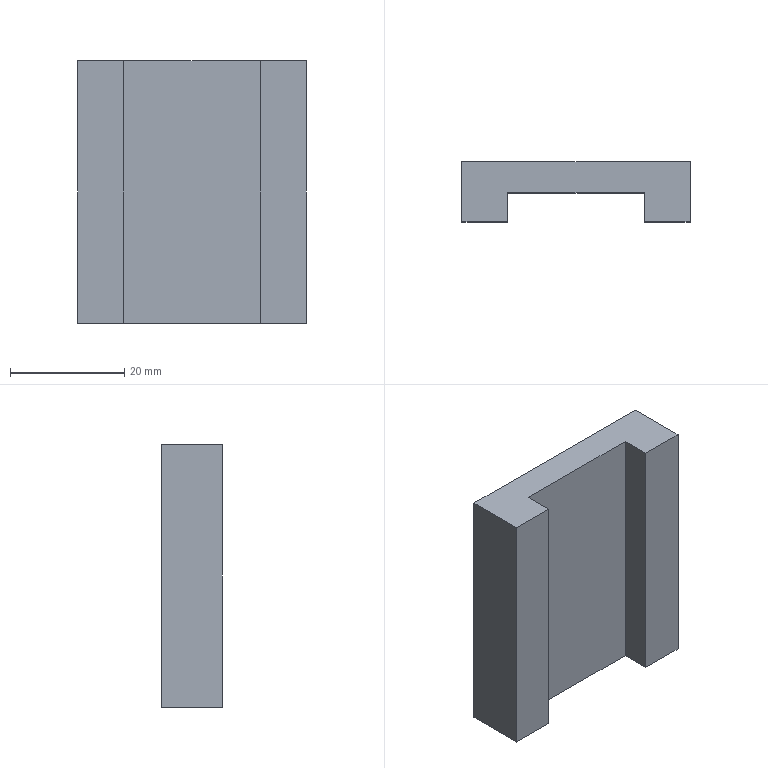Part | STEP file | 11-MGW12C11 | 1 solid | 26 faces | box 40 x 10.6 x 46 mm | volume 13798 mm3 | plane 10 | cone 8 | cylinder 8 | commonest cylinder face diameters 2.5 x8
STEP:
#1=CARTESIAN_POINT('',(-45.352,-1.993,15.5));
#2=VERTEX_POINT('',#1);
#3=CARTESIAN_POINT('',(-45.352,-1.242,16.75));
#4=VERTEX_POINT('',#3);
#5=CARTESIAN_POINT('',(-45.352,-1.242,16.75));
#6=DIRECTION('',(0.,0.515,0.8572));
#7=VECTOR('',#6,1000.);
#8=LINE('',#5,#7);
#9=EDGE_CURVE('',#2,#4,#8,.T.);
#10=ORIENTED_EDGE('',*,*,#9,.F.);
#11=CARTESIAN_POINT('',(-45.352,-1.242,14.25));
#12=VERTEX_POINT('',#11);
#13=CARTESIAN_POINT('',(-45.352,-1.242,14.25));
#14=DIRECTION('',(0.,0.515,-0.8572));
#15=VECTOR('',#14,1000.);
#16=LINE('',#13,#15);
#17=EDGE_CURVE('',#2,#12,#16,.T.);
#18=ORIENTED_EDGE('',*,*,#17,.T.);
#19=CARTESIAN_POINT('',(-45.352,-1.242,15.5));
#20=DIRECTION('',(0.,1.,0.));
#21=DIRECTION('',(0.,0.,1.));
#22=AXIS2_PLACEMENT_3D('',#19,#20,#21);
#23=CIRCLE('',#22,1.25);
#24=EDGE_CURVE('',#12,#4,#23,.T.);
#25=ORIENTED_EDGE('',*,*,#24,.T.);
#26=EDGE_LOOP('',(#10,#18,#25));
#27=FACE_OUTER_BOUND('',#26,.T.);
#28=CARTESIAN_POINT('',(-45.352,-1.242,15.5));
#29=DIRECTION('',(0.,1.,0.));
#30=DIRECTION('',(0.,0.,1.));
#31=AXIS2_PLACEMENT_3D('',#28,#29,#30);
#32=CONICAL_SURFACE('',#31,1.25,1.03);
#33=ADVANCED_FACE('',(#27),#32,.F.);
#34=ORIENTED_EDGE('',*,*,#24,.F.);
#35=CARTESIAN_POINT('',(-45.352,2.358,14.25));
#36=VERTEX_POINT('',#35);
#37=CARTESIAN_POINT('',(-45.352,2.358,14.25));
#38=DIRECTION('',(0.,1.,0.));
#39=VECTOR('',#38,1000.);
#40=LINE('',#37,#39);
#41=EDGE_CURVE('',#12,#36,#40,.T.);
#42=ORIENTED_EDGE('',*,*,#41,.T.);
#43=CARTESIAN_POINT('',(-45.352,2.358,16.75));
#44=VERTEX_POINT('',#43);
#45=CARTESIAN_POINT('',(-45.352,2.358,15.5));
#46=DIRECTION('',(0.,1.,0.));
#47=DIRECTION('',(0.,0.,1.));
#48=AXIS2_PLACEMENT_3D('',#45,#46,#47);
#49=CIRCLE('',#48,1.25);
#50=EDGE_CURVE('',#36,#44,#49,.T.);
#51=ORIENTED_EDGE('',*,*,#50,.T.);
#52=CARTESIAN_POINT('',(-45.352,2.358,16.75));
#53=DIRECTION('',(0.,1.,0.));
#54=VECTOR('',#53,1000.);
#55=LINE('',#52,#54);
#56=EDGE_CURVE('',#4,#44,#55,.T.);
#57=ORIENTED_EDGE('',*,*,#56,.F.);
#58=EDGE_LOOP('',(#34,#42,#51,#57));
#59=FACE_OUTER_BOUND('',#58,.T.);
#60=CARTESIAN_POINT('',(-45.352,2.358,15.5));
#61=DIRECTION('',(0.,1.,0.));
#62=DIRECTION('',(0.,0.,1.));
#63=AXIS2_PLACEMENT_3D('',#60,#61,#62);
#64=CYLINDRICAL_SURFACE('',#63,1.25);
#65=ADVANCED_FACE('',(#59),#64,.F.);
#66=CARTESIAN_POINT('',(-17.352,-1.993,15.5));
#67=VERTEX_POINT('',#66);
#68=CARTESIAN_POINT('',(-17.352,-1.242,16.75));
#69=VERTEX_POINT('',#68);
#70=CARTESIAN_POINT('',(-17.352,-1.242,16.75));
#71=DIRECTION('',(0.,0.515,0.8572));
#72=VECTOR('',#71,1000.);
#73=LINE('',#70,#72);
#74=EDGE_CURVE('',#67,#69,#73,.T.);
#75=ORIENTED_EDGE('',*,*,#74,.F.);
#76=CARTESIAN_POINT('',(-17.352,-1.242,14.25));
#77=VERTEX_POINT('',#76);
#78=CARTESIAN_POINT('',(-17.352,-1.242,14.25));
#79=DIRECTION('',(0.,0.515,-0.8572));
#80=VECTOR('',#79,1000.);
#81=LINE('',#78,#80);
#82=EDGE_CURVE('',#67,#77,#81,.T.);
#83=ORIENTED_EDGE('',*,*,#82,.T.);
#84=CARTESIAN_POINT('',(-17.352,-1.242,15.5));
#85=DIRECTION('',(0.,1.,0.));
#86=DIRECTION('',(0.,0.,1.));
#87=AXIS2_PLACEMENT_3D('',#84,#85,#86);
#88=CIRCLE('',#87,1.25);
#89=EDGE_CURVE('',#77,#69,#88,.T.);
#90=ORIENTED_EDGE('',*,*,#89,.T.);
#91=EDGE_LOOP('',(#75,#83,#90));
#92=FACE_OUTER_BOUND('',#91,.T.);
#93=CARTESIAN_POINT('',(-17.352,-1.242,15.5));
#94=DIRECTION('',(0.,1.,0.));
#95=DIRECTION('',(0.,0.,1.));
#96=AXIS2_PLACEMENT_3D('',#93,#94,#95);
#97=CONICAL_SURFACE('',#96,1.25,1.03);
#98=ADVANCED_FACE('',(#92),#97,.F.);
#99=ORIENTED_EDGE('',*,*,#89,.F.);
#100=CARTESIAN_POINT('',(-17.352,2.358,14.25));
#101=VERTEX_POINT('',#100);
#102=CARTESIAN_POINT('',(-17.352,2.358,14.25));
#103=DIRECTION('',(0.,1.,0.));
#104=VECTOR('',#103,1000.);
#105=LINE('',#102,#104);
#106=EDGE_CURVE('',#77,#101,#105,.T.);
#107=ORIENTED_EDGE('',*,*,#106,.T.);
#108=CARTESIAN_POINT('',(-17.352,2.358,16.75));
#109=VERTEX_POINT('',#108);
#110=CARTESIAN_POINT('',(-17.352,2.358,15.5));
#111=DIRECTION('',(0.,1.,0.));
#112=DIRECTION('',(0.,0.,1.));
#113=AXIS2_PLACEMENT_3D('',#110,#111,#112);
#114=CIRCLE('',#113,1.25);
#115=EDGE_CURVE('',#101,#109,#114,.T.);
#116=ORIENTED_EDGE('',*,*,#115,.T.);
#117=CARTESIAN_POINT('',(-17.352,2.358,16.75));
#118=DIRECTION('',(0.,1.,0.));
#119=VECTOR('',#118,1000.);
#120=LINE('',#117,#119);
#121=EDGE_CURVE('',#69,#109,#120,.T.);
#122=ORIENTED_EDGE('',*,*,#121,.F.);
#123=EDGE_LOOP('',(#99,#107,#116,#122));
#124=FACE_OUTER_BOUND('',#123,.T.);
#125=CARTESIAN_POINT('',(-17.352,2.358,15.5));
#126=DIRECTION('',(0.,1.,0.));
#127=DIRECTION('',(0.,0.,1.));
#128=AXIS2_PLACEMENT_3D('',#125,#126,#127);
#129=CYLINDRICAL_SURFACE('',#128,1.25);
#130=ADVANCED_FACE('',(#124),#129,.F.);
#131=CARTESIAN_POINT('',(-45.352,-1.242,29.25));
#132=VERTEX_POINT('',#131);
#133=CARTESIAN_POINT('',(-45.352,-1.242,31.75));
#134=VERTEX_POINT('',#133);
#135=CARTESIAN_POINT('',(-45.352,-1.242,30.5));
#136=DIRECTION('',(0.,1.,0.));
#137=DIRECTION('',(0.,0.,1.));
#138=AXIS2_PLACEMENT_3D('',#135,#136,#137);
#139=CIRCLE('',#138,1.25);
#140=EDGE_CURVE('',#132,#134,#139,.T.);
#141=ORIENTED_EDGE('',*,*,#140,.F.);
#142=CARTESIAN_POINT('',(-45.352,2.358,29.25));
#143=VERTEX_POINT('',#142);
#144=CARTESIAN_POINT('',(-45.352,2.358,29.25));
#145=DIRECTION('',(0.,1.,0.));
#146=VECTOR('',#145,1000.);
#147=LINE('',#144,#146);
#148=EDGE_CURVE('',#132,#143,#147,.T.);
#149=ORIENTED_EDGE('',*,*,#148,.T.);
#150=CARTESIAN_POINT('',(-45.352,2.358,31.75));
#151=VERTEX_POINT('',#150);
#152=CARTESIAN_POINT('',(-45.352,2.358,30.5));
#153=DIRECTION('',(0.,1.,0.));
#154=DIRECTION('',(0.,0.,1.));
#155=AXIS2_PLACEMENT_3D('',#152,#153,#154);
#156=CIRCLE('',#155,1.25);
#157=EDGE_CURVE('',#143,#151,#156,.T.);
#158=ORIENTED_EDGE('',*,*,#157,.T.);
#159=CARTESIAN_POINT('',(-45.352,2.358,31.75));
#160=DIRECTION('',(0.,1.,0.));
#161=VECTOR('',#160,1000.);
#162=LINE('',#159,#161);
#163=EDGE_CURVE('',#134,#151,#162,.T.);
#164=ORIENTED_EDGE('',*,*,#163,.F.);
#165=EDGE_LOOP('',(#141,#149,#158,#164));
#166=FACE_OUTER_BOUND('',#165,.T.);
#167=CARTESIAN_POINT('',(-45.352,2.358,30.5));
#168=DIRECTION('',(0.,1.,0.));
#169=DIRECTION('',(0.,0.,1.));
#170=AXIS2_PLACEMENT_3D('',#167,#168,#169);
#171=CYLINDRICAL_SURFACE('',#170,1.25);
#172=ADVANCED_FACE('',(#166),#171,.F.);
#173=CARTESIAN_POINT('',(-45.352,-1.993,30.5));
#174=VERTEX_POINT('',#173);
#175=CARTESIAN_POINT('',(-45.352,-1.242,31.75));
#176=DIRECTION('',(0.,0.515,0.8572));
#177=VECTOR('',#176,1000.);
#178=LINE('',#175,#177);
#179=EDGE_CURVE('',#174,#134,#178,.T.);
#180=ORIENTED_EDGE('',*,*,#179,.F.);
#181=CARTESIAN_POINT('',(-45.352,-1.242,29.25));
#182=DIRECTION('',(0.,0.515,-0.8572));
#183=VECTOR('',#182,1000.);
#184=LINE('',#181,#183);
#185=EDGE_CURVE('',#174,#132,#184,.T.);
#186=ORIENTED_EDGE('',*,*,#185,.T.);
#187=ORIENTED_EDGE('',*,*,#140,.T.);
#188=EDGE_LOOP('',(#180,#186,#187));
#189=FACE_OUTER_BOUND('',#188,.T.);
#190=CARTESIAN_POINT('',(-45.352,-1.242,30.5));
#191=DIRECTION('',(0.,1.,0.));
#192=DIRECTION('',(0.,0.,1.));
#193=AXIS2_PLACEMENT_3D('',#190,#191,#192);
#194=CONICAL_SURFACE('',#193,1.25,1.03);
#195=ADVANCED_FACE('',(#189),#194,.F.);
#196=CARTESIAN_POINT('',(-17.352,-1.242,29.25));
#197=VERTEX_POINT('',#196);
#198=CARTESIAN_POINT('',(-17.352,-1.242,31.75));
#199=VERTEX_POINT('',#198);
#200=CARTESIAN_POINT('',(-17.352,-1.242,30.5));
#201=DIRECTION('',(0.,1.,0.));
#202=DIRECTION('',(0.,0.,1.));
#203=AXIS2_PLACEMENT_3D('',#200,#201,#202);
#204=CIRCLE('',#203,1.25);
#205=EDGE_CURVE('',#197,#199,#204,.T.);
#206=ORIENTED_EDGE('',*,*,#205,.F.);
#207=CARTESIAN_POINT('',(-17.352,2.358,29.25));
#208=VERTEX_POINT('',#207);
#209=CARTESIAN_POINT('',(-17.352,2.358,29.25));
#210=DIRECTION('',(0.,1.,0.));
#211=VECTOR('',#210,1000.);
#212=LINE('',#209,#211);
#213=EDGE_CURVE('',#197,#208,#212,.T.);
#214=ORIENTED_EDGE('',*,*,#213,.T.);
#215=CARTESIAN_POINT('',(-17.352,2.358,31.75));
#216=VERTEX_POINT('',#215);
#217=CARTESIAN_POINT('',(-17.352,2.358,30.5));
#218=DIRECTION('',(0.,1.,0.));
#219=DIRECTION('',(0.,0.,1.));
#220=AXIS2_PLACEMENT_3D('',#217,#218,#219);
#221=CIRCLE('',#220,1.25);
#222=EDGE_CURVE('',#208,#216,#221,.T.);
#223=ORIENTED_EDGE('',*,*,#222,.T.);
#224=CARTESIAN_POINT('',(-17.352,2.358,31.75));
#225=DIRECTION('',(0.,1.,0.));
#226=VECTOR('',#225,1000.);
#227=LINE('',#224,#226);
#228=EDGE_CURVE('',#199,#216,#227,.T.);
#229=ORIENTED_EDGE('',*,*,#228,.F.);
#230=EDGE_LOOP('',(#206,#214,#223,#229));
#231=FACE_OUTER_BOUND('',#230,.T.);
#232=CARTESIAN_POINT('',(-17.352,2.358,30.5));
#233=DIRECTION('',(0.,1.,0.));
#234=DIRECTION('',(0.,0.,1.));
#235=AXIS2_PLACEMENT_3D('',#232,#233,#234);
#236=CYLINDRICAL_SURFACE('',#235,1.25);
#237=ADVANCED_FACE('',(#231),#236,.F.);
#238=CARTESIAN_POINT('',(-17.352,-1.993,30.5));
#239=VERTEX_POINT('',#238);
#240=CARTESIAN_POINT('',(-17.352,-1.242,31.75));
#241=DIRECTION('',(0.,0.515,0.8572));
#242=VECTOR('',#241,1000.);
#243=LINE('',#240,#242);
#244=EDGE_CURVE('',#239,#199,#243,.T.);
#245=ORIENTED_EDGE('',*,*,#244,.F.);
#246=CARTESIAN_POINT('',(-17.352,-1.242,29.25));
#247=DIRECTION('',(0.,0.515,-0.8572));
#248=VECTOR('',#247,1000.);
#249=LINE('',#246,#248);
#250=EDGE_CURVE('',#239,#197,#249,.T.);
#251=ORIENTED_EDGE('',*,*,#250,.T.);
#252=ORIENTED_EDGE('',*,*,#205,.T.);
#253=EDGE_LOOP('',(#245,#251,#252));
#254=FACE_OUTER_BOUND('',#253,.T.);
#255=CARTESIAN_POINT('',(-17.352,-1.242,30.5));
#256=DIRECTION('',(0.,1.,0.));
#257=DIRECTION('',(0.,0.,1.));
#258=AXIS2_PLACEMENT_3D('',#255,#256,#257);
#259=CONICAL_SURFACE('',#258,1.25,1.03);
#260=ADVANCED_FACE('',(#254),#259,.F.);
#261=CARTESIAN_POINT('',(-51.352,-8.242,0.));
#262=VERTEX_POINT('',#261);
#263=CARTESIAN_POINT('',(-43.352,-8.242,0.));
#264=VERTEX_POINT('',#263);
#265=CARTESIAN_POINT('',(-51.352,-8.242,0.));
#266=DIRECTION('',(1.,0.,0.));
#267=VECTOR('',#266,1000.);
#268=LINE('',#265,#267);
#269=EDGE_CURVE('',#262,#264,#268,.T.);
#270=ORIENTED_EDGE('',*,*,#269,.T.);
#271=CARTESIAN_POINT('',(-43.352,-8.242,46.));
#272=VERTEX_POINT('',#271);
#273=CARTESIAN_POINT('',(-43.352,-8.242,46.));
#274=DIRECTION('',(0.,0.,-1.));
#275=VECTOR('',#274,1000.);
#276=LINE('',#273,#275);
#277=EDGE_CURVE('',#272,#264,#276,.T.);
#278=ORIENTED_EDGE('',*,*,#277,.F.);
#279=CARTESIAN_POINT('',(-51.352,-8.242,46.));
#280=VERTEX_POINT('',#279);
#281=CARTESIAN_POINT('',(-51.352,-8.242,46.));
#282=DIRECTION('',(1.,0.,0.));
#283=VECTOR('',#282,1000.);
#284=LINE('',#281,#283);
#285=EDGE_CURVE('',#280,#272,#284,.T.);
#286=ORIENTED_EDGE('',*,*,#285,.F.);
#287=CARTESIAN_POINT('',(-51.352,-8.242,46.));
#288=DIRECTION('',(0.,0.,-1.));
#289=VECTOR('',#288,1000.);
#290=LINE('',#287,#289);
#291=EDGE_CURVE('',#280,#262,#290,.T.);
#292=ORIENTED_EDGE('',*,*,#291,.T.);
#293=EDGE_LOOP('',(#270,#278,#286,#292));
#294=FACE_OUTER_BOUND('',#293,.T.);
#295=CARTESIAN_POINT('',(-51.352,-8.242,46.));
#296=DIRECTION('',(0.,1.,0.));
#297=DIRECTION('',(-1.,0.,0.));
#298=AXIS2_PLACEMENT_3D('',#295,#296,#297);
#299=PLANE('',#298);
#300=ADVANCED_FACE('',(#294),#299,.F.);
#301=CARTESIAN_POINT('',(-51.352,2.358,0.));
#302=VERTEX_POINT('',#301);
#303=CARTESIAN_POINT('',(-51.352,2.358,0.));
#304=DIRECTION('',(0.,-1.,0.));
#305=VECTOR('',#304,1000.);
#306=LINE('',#303,#305);
#307=EDGE_CURVE('',#302,#262,#306,.T.);
#308=ORIENTED_EDGE('',*,*,#307,.T.);
#309=ORIENTED_EDGE('',*,*,#291,.F.);
#310=CARTESIAN_POINT('',(-51.352,2.358,46.));
#311=VERTEX_POINT('',#310);
#312=CARTESIAN_POINT('',(-51.352,2.358,46.));
#313=DIRECTION('',(0.,-1.,0.));
#314=VECTOR('',#313,1000.);
#315=LINE('',#312,#314);
#316=EDGE_CURVE('',#311,#280,#315,.T.);
#317=ORIENTED_EDGE('',*,*,#316,.F.);
#318=CARTESIAN_POINT('',(-51.352,2.358,46.));
#319=DIRECTION('',(0.,0.,-1.));
#320=VECTOR('',#319,1000.);
#321=LINE('',#318,#320);
#322=EDGE_CURVE('',#311,#302,#321,.T.);
#323=ORIENTED_EDGE('',*,*,#322,.T.);
#324=EDGE_LOOP('',(#308,#309,#317,#323));
#325=FACE_OUTER_BOUND('',#324,.T.);
#326=CARTESIAN_POINT('',(-51.352,2.358,46.));
#327=DIRECTION('',(1.,0.,0.));
#328=DIRECTION('',(0.,1.,0.));
#329=AXIS2_PLACEMENT_3D('',#326,#327,#328);
#330=PLANE('',#329);
#331=ADVANCED_FACE('',(#325),#330,.F.);
#332=CARTESIAN_POINT('',(-19.352,-8.242,46.));
#333=VERTEX_POINT('',#332);
#334=CARTESIAN_POINT('',(-11.352,-8.242,46.));
#335=VERTEX_POINT('',#334);
#336=CARTESIAN_POINT('',(-51.352,-8.242,46.));
#337=DIRECTION('',(1.,0.,0.));
#338=VECTOR('',#337,1000.);
#339=LINE('',#336,#338);
#340=EDGE_CURVE('',#333,#335,#339,.T.);
#341=ORIENTED_EDGE('',*,*,#340,.F.);
#342=CARTESIAN_POINT('',(-19.352,-8.242,0.));
#343=VERTEX_POINT('',#342);
#344=CARTESIAN_POINT('',(-19.352,-8.242,46.));
#345=DIRECTION('',(0.,0.,1.));
#346=VECTOR('',#345,1000.);
#347=LINE('',#344,#346);
#348=EDGE_CURVE('',#343,#333,#347,.T.);
#349=ORIENTED_EDGE('',*,*,#348,.F.);
#350=CARTESIAN_POINT('',(-11.352,-8.242,0.));
#351=VERTEX_POINT('',#350);
#352=CARTESIAN_POINT('',(-51.352,-8.242,0.));
#353=DIRECTION('',(1.,0.,0.));
#354=VECTOR('',#353,1000.);
#355=LINE('',#352,#354);
#356=EDGE_CURVE('',#343,#351,#355,.T.);
#357=ORIENTED_EDGE('',*,*,#356,.T.);
#358=CARTESIAN_POINT('',(-11.352,-8.242,46.));
#359=DIRECTION('',(0.,0.,-1.));
#360=VECTOR('',#359,1000.);
#361=LINE('',#358,#360);
#362=EDGE_CURVE('',#335,#351,#361,.T.);
#363=ORIENTED_EDGE('',*,*,#362,.F.);
#364=EDGE_LOOP('',(#341,#349,#357,#363));
#365=FACE_OUTER_BOUND('',#364,.T.);
#366=CARTESIAN_POINT('',(-51.352,-8.242,46.));
#367=DIRECTION('',(0.,1.,0.));
#368=DIRECTION('',(-1.,0.,0.));
#369=AXIS2_PLACEMENT_3D('',#366,#367,#368);
#370=PLANE('',#369);
#371=ADVANCED_FACE('',(#365),#370,.F.);
#372=CARTESIAN_POINT('',(-11.352,2.358,0.));
#373=VERTEX_POINT('',#372);
#374=CARTESIAN_POINT('',(-11.352,2.358,0.));
#375=DIRECTION('',(0.,1.,0.));
#376=VECTOR('',#375,1000.);
#377=LINE('',#374,#376);
#378=EDGE_CURVE('',#351,#373,#377,.T.);
#379=ORIENTED_EDGE('',*,*,#378,.T.);
#380=CARTESIAN_POINT('',(-11.352,2.358,46.));
#381=VERTEX_POINT('',#380);
#382=CARTESIAN_POINT('',(-11.352,2.358,46.));
#383=DIRECTION('',(0.,0.,-1.));
#384=VECTOR('',#383,1000.);
#385=LINE('',#382,#384);
#386=EDGE_CURVE('',#381,#373,#385,.T.);
#387=ORIENTED_EDGE('',*,*,#386,.F.);
#388=CARTESIAN_POINT('',(-11.352,2.358,46.));
#389=DIRECTION('',(0.,1.,0.));
#390=VECTOR('',#389,1000.);
#391=LINE('',#388,#390);
#392=EDGE_CURVE('',#335,#381,#391,.T.);
#393=ORIENTED_EDGE('',*,*,#392,.F.);
#394=ORIENTED_EDGE('',*,*,#362,.T.);
#395=EDGE_LOOP('',(#379,#387,#393,#394));
#396=FACE_OUTER_BOUND('',#395,.T.);
#397=CARTESIAN_POINT('',(-11.352,2.358,46.));
#398=DIRECTION('',(-1.,0.,0.));
#399=DIRECTION('',(0.,0.,1.));
#400=AXIS2_PLACEMENT_3D('',#397,#398,#399);
#401=PLANE('',#400);
#402=ADVANCED_FACE('',(#396),#401,.F.);
#403=CARTESIAN_POINT('',(-45.352,2.358,30.5));
#404=DIRECTION('',(0.,1.,0.));
#405=DIRECTION('',(0.,0.,1.));
#406=AXIS2_PLACEMENT_3D('',#403,#404,#405);
#407=CIRCLE('',#406,1.25);
#408=EDGE_CURVE('',#151,#143,#407,.T.);
#409=ORIENTED_EDGE('',*,*,#408,.F.);
#410=ORIENTED_EDGE('',*,*,#157,.F.);
#411=EDGE_LOOP('',(#409,#410));
#412=FACE_BOUND('',#411,.T.);
#413=CARTESIAN_POINT('',(-17.352,2.358,30.5));
#414=DIRECTION('',(0.,1.,0.));
#415=DIRECTION('',(0.,0.,1.));
#416=AXIS2_PLACEMENT_3D('',#413,#414,#415);
#417=CIRCLE('',#416,1.25);
#418=EDGE_CURVE('',#216,#208,#417,.T.);
#419=ORIENTED_EDGE('',*,*,#418,.F.);
#420=ORIENTED_EDGE('',*,*,#222,.F.);
#421=EDGE_LOOP('',(#419,#420));
#422=FACE_BOUND('',#421,.T.);
#423=CARTESIAN_POINT('',(-51.352,2.358,0.));
#424=DIRECTION('',(-1.,0.,0.));
#425=VECTOR('',#424,1000.);
#426=LINE('',#423,#425);
#427=EDGE_CURVE('',#373,#302,#426,.T.);
#428=ORIENTED_EDGE('',*,*,#427,.T.);
#429=ORIENTED_EDGE('',*,*,#322,.F.);
#430=CARTESIAN_POINT('',(-51.352,2.358,46.));
#431=DIRECTION('',(-1.,0.,0.));
#432=VECTOR('',#431,1000.);
#433=LINE('',#430,#432);
#434=EDGE_CURVE('',#381,#311,#433,.T.);
#435=ORIENTED_EDGE('',*,*,#434,.F.);
#436=ORIENTED_EDGE('',*,*,#386,.T.);
#437=EDGE_LOOP('',(#428,#429,#435,#436));
#438=FACE_OUTER_BOUND('',#437,.T.);
#439=CARTESIAN_POINT('',(-17.352,2.358,15.5));
#440=DIRECTION('',(0.,1.,0.));
#441=DIRECTION('',(0.,0.,1.));
#442=AXIS2_PLACEMENT_3D('',#439,#440,#441);
#443=CIRCLE('',#442,1.25);
#444=EDGE_CURVE('',#109,#101,#443,.T.);
#445=ORIENTED_EDGE('',*,*,#444,.F.);
#446=ORIENTED_EDGE('',*,*,#115,.F.);
#447=EDGE_LOOP('',(#445,#446));
#448=FACE_BOUND('',#447,.T.);
#449=CARTESIAN_POINT('',(-45.352,2.358,15.5));
#450=DIRECTION('',(0.,1.,0.));
#451=DIRECTION('',(0.,0.,1.));
#452=AXIS2_PLACEMENT_3D('',#449,#450,#451);
#453=CIRCLE('',#452,1.25);
#454=EDGE_CURVE('',#44,#36,#453,.T.);
#455=ORIENTED_EDGE('',*,*,#454,.F.);
#456=ORIENTED_EDGE('',*,*,#50,.F.);
#457=EDGE_LOOP('',(#455,#456));
#458=FACE_BOUND('',#457,.T.);
#459=CARTESIAN_POINT('',(-51.352,2.358,46.));
#460=DIRECTION('',(0.,-1.,0.));
#461=DIRECTION('',(0.,0.,-1.));
#462=AXIS2_PLACEMENT_3D('',#459,#460,#461);
#463=PLANE('',#462);
#464=ADVANCED_FACE('',(#412,#422,#438,#448,#458),#463,.F.);
#465=CARTESIAN_POINT('',(-43.352,-3.142,46.));
#466=VERTEX_POINT('',#465);
#467=CARTESIAN_POINT('',(-43.352,-3.142,46.));
#468=DIRECTION('',(0.,-1.,0.));
#469=VECTOR('',#468,1000.);
#470=LINE('',#467,#469);
#471=EDGE_CURVE('',#466,#272,#470,.T.);
#472=ORIENTED_EDGE('',*,*,#471,.F.);
#473=CARTESIAN_POINT('',(-19.352,-3.142,46.));
#474=VERTEX_POINT('',#473);
#475=CARTESIAN_POINT('',(-43.352,-3.142,46.));
#476=DIRECTION('',(-1.,0.,0.));
#477=VECTOR('',#476,1000.);
#478=LINE('',#475,#477);
#479=EDGE_CURVE('',#474,#466,#478,.T.);
#480=ORIENTED_EDGE('',*,*,#479,.F.);
#481=CARTESIAN_POINT('',(-19.352,-3.142,46.));
#482=DIRECTION('',(0.,-1.,0.));
#483=VECTOR('',#482,1000.);
#484=LINE('',#481,#483);
#485=EDGE_CURVE('',#474,#333,#484,.T.);
#486=ORIENTED_EDGE('',*,*,#485,.T.);
#487=ORIENTED_EDGE('',*,*,#340,.T.);
#488=ORIENTED_EDGE('',*,*,#392,.T.);
#489=ORIENTED_EDGE('',*,*,#434,.T.);
#490=ORIENTED_EDGE('',*,*,#316,.T.);
#491=ORIENTED_EDGE('',*,*,#285,.T.);
#492=EDGE_LOOP('',(#472,#480,#486,#487,#488,#489,#490,#491));
#493=FACE_OUTER_BOUND('',#492,.T.);
#494=CARTESIAN_POINT('',(-51.352,-8.242,46.));
#495=DIRECTION('',(0.,0.,1.));
#496=DIRECTION('',(1.,0.,0.));
#497=AXIS2_PLACEMENT_3D('',#494,#495,#496);
#498=PLANE('',#497);
#499=ADVANCED_FACE('',(#493),#498,.T.);
#500=CARTESIAN_POINT('',(-43.352,-3.142,0.));
#501=VERTEX_POINT('',#500);
#502=CARTESIAN_POINT('',(-19.352,-3.142,0.));
#503=VERTEX_POINT('',#502);
#504=CARTESIAN_POINT('',(-43.352,-3.142,0.));
#505=DIRECTION('',(1.,0.,0.));
#506=VECTOR('',#505,1000.);
#507=LINE('',#504,#506);
#508=EDGE_CURVE('',#501,#503,#507,.T.);
#509=ORIENTED_EDGE('',*,*,#508,.F.);
#510=CARTESIAN_POINT('',(-43.352,-3.142,0.));
#511=DIRECTION('',(0.,-1.,0.));
#512=VECTOR('',#511,1000.);
#513=LINE('',#510,#512);
#514=EDGE_CURVE('',#501,#264,#513,.T.);
#515=ORIENTED_EDGE('',*,*,#514,.T.);
#516=ORIENTED_EDGE('',*,*,#269,.F.);
#517=ORIENTED_EDGE('',*,*,#307,.F.);
#518=ORIENTED_EDGE('',*,*,#427,.F.);
#519=ORIENTED_EDGE('',*,*,#378,.F.);
#520=ORIENTED_EDGE('',*,*,#356,.F.);
#521=CARTESIAN_POINT('',(-19.352,-3.142,0.));
#522=DIRECTION('',(0.,-1.,0.));
#523=VECTOR('',#522,1000.);
#524=LINE('',#521,#523);
#525=EDGE_CURVE('',#503,#343,#524,.T.);
#526=ORIENTED_EDGE('',*,*,#525,.F.);
#527=EDGE_LOOP('',(#509,#515,#516,#517,#518,#519,#520,#526));
#528=FACE_OUTER_BOUND('',#527,.T.);
#529=CARTESIAN_POINT('',(-51.352,-8.242,0.));
#530=DIRECTION('',(0.,0.,1.));
#531=DIRECTION('',(1.,0.,0.));
#532=AXIS2_PLACEMENT_3D('',#529,#530,#531);
#533=PLANE('',#532);
#534=ADVANCED_FACE('',(#528),#533,.F.);
#535=ORIENTED_EDGE('',*,*,#277,.T.);
#536=ORIENTED_EDGE('',*,*,#514,.F.);
#537=CARTESIAN_POINT('',(-43.352,-3.142,46.));
#538=DIRECTION('',(0.,0.,-1.));
#539=VECTOR('',#538,1000.);
#540=LINE('',#537,#539);
#541=EDGE_CURVE('',#466,#501,#540,.T.);
#542=ORIENTED_EDGE('',*,*,#541,.F.);
#543=ORIENTED_EDGE('',*,*,#471,.T.);
#544=EDGE_LOOP('',(#535,#536,#542,#543));
#545=FACE_OUTER_BOUND('',#544,.T.);
#546=CARTESIAN_POINT('',(-43.352,-3.142,46.));
#547=DIRECTION('',(-1.,0.,0.));
#548=DIRECTION('',(0.,0.,1.));
#549=AXIS2_PLACEMENT_3D('',#546,#547,#548);
#550=PLANE('',#549);
#551=ADVANCED_FACE('',(#545),#550,.F.);
#552=ORIENTED_EDGE('',*,*,#348,.T.);
#553=ORIENTED_EDGE('',*,*,#485,.F.);
#554=CARTESIAN_POINT('',(-19.352,-3.142,46.));
#555=DIRECTION('',(0.,0.,1.));
#556=VECTOR('',#555,1000.);
#557=LINE('',#554,#556);
#558=EDGE_CURVE('',#503,#474,#557,.T.);
#559=ORIENTED_EDGE('',*,*,#558,.F.);
#560=ORIENTED_EDGE('',*,*,#525,.T.);
#561=EDGE_LOOP('',(#552,#553,#559,#560));
#562=FACE_OUTER_BOUND('',#561,.T.);
#563=CARTESIAN_POINT('',(-19.352,-3.142,46.));
#564=DIRECTION('',(1.,0.,0.));
#565=DIRECTION('',(0.,0.,-1.));
#566=AXIS2_PLACEMENT_3D('',#563,#564,#565);
#567=PLANE('',#566);
#568=ADVANCED_FACE('',(#562),#567,.F.);
#569=ORIENTED_EDGE('',*,*,#541,.T.);
#570=ORIENTED_EDGE('',*,*,#508,.T.);
#571=ORIENTED_EDGE('',*,*,#558,.T.);
#572=ORIENTED_EDGE('',*,*,#479,.T.);
#573=EDGE_LOOP('',(#569,#570,#571,#572));
#574=FACE_OUTER_BOUND('',#573,.T.);
#575=CARTESIAN_POINT('',(-43.352,-3.142,0.));
#576=DIRECTION('',(0.,-1.,0.));
#577=DIRECTION('',(1.,0.,0.));
#578=AXIS2_PLACEMENT_3D('',#575,#576,#577);
#579=PLANE('',#578);
#580=ADVANCED_FACE('',(#574),#579,.T.);
#581=ORIENTED_EDGE('',*,*,#250,.F.);
#582=ORIENTED_EDGE('',*,*,#244,.T.);
#583=CARTESIAN_POINT('',(-17.352,-1.242,30.5));
#584=DIRECTION('',(0.,1.,0.));
#585=DIRECTION('',(0.,0.,1.));
#586=AXIS2_PLACEMENT_3D('',#583,#584,#585);
#587=CIRCLE('',#586,1.25);
#588=EDGE_CURVE('',#199,#197,#587,.T.);
#589=ORIENTED_EDGE('',*,*,#588,.T.);
#590=EDGE_LOOP('',(#581,#582,#589));
#591=FACE_OUTER_BOUND('',#590,.T.);
#592=CARTESIAN_POINT('',(-17.352,-1.242,30.5));
#593=DIRECTION('',(0.,1.,0.));
#594=DIRECTION('',(0.,0.,1.));
#595=AXIS2_PLACEMENT_3D('',#592,#593,#594);
#596=CONICAL_SURFACE('',#595,1.25,1.03);
#597=ADVANCED_FACE('',(#591),#596,.F.);
#598=ORIENTED_EDGE('',*,*,#213,.F.);
#599=ORIENTED_EDGE('',*,*,#588,.F.);
#600=ORIENTED_EDGE('',*,*,#228,.T.);
#601=ORIENTED_EDGE('',*,*,#418,.T.);
#602=EDGE_LOOP('',(#598,#599,#600,#601));
#603=FACE_OUTER_BOUND('',#602,.T.);
#604=CARTESIAN_POINT('',(-17.352,2.358,30.5));
#605=DIRECTION('',(0.,1.,0.));
#606=DIRECTION('',(0.,0.,1.));
#607=AXIS2_PLACEMENT_3D('',#604,#605,#606);
#608=CYLINDRICAL_SURFACE('',#607,1.25);
#609=ADVANCED_FACE('',(#603),#608,.F.);
#610=ORIENTED_EDGE('',*,*,#148,.F.);
#611=CARTESIAN_POINT('',(-45.352,-1.242,30.5));
#612=DIRECTION('',(0.,1.,0.));
#613=DIRECTION('',(0.,0.,1.));
#614=AXIS2_PLACEMENT_3D('',#611,#612,#613);
#615=CIRCLE('',#614,1.25);
#616=EDGE_CURVE('',#134,#132,#615,.T.);
#617=ORIENTED_EDGE('',*,*,#616,.F.);
#618=ORIENTED_EDGE('',*,*,#163,.T.);
#619=ORIENTED_EDGE('',*,*,#408,.T.);
#620=EDGE_LOOP('',(#610,#617,#618,#619));
#621=FACE_OUTER_BOUND('',#620,.T.);
#622=CARTESIAN_POINT('',(-45.352,2.358,30.5));
#623=DIRECTION('',(0.,1.,0.));
#624=DIRECTION('',(0.,0.,1.));
#625=AXIS2_PLACEMENT_3D('',#622,#623,#624);
#626=CYLINDRICAL_SURFACE('',#625,1.25);
#627=ADVANCED_FACE('',(#621),#626,.F.);
#628=ORIENTED_EDGE('',*,*,#185,.F.);
#629=ORIENTED_EDGE('',*,*,#179,.T.);
#630=ORIENTED_EDGE('',*,*,#616,.T.);
#631=EDGE_LOOP('',(#628,#629,#630));
#632=FACE_OUTER_BOUND('',#631,.T.);
#633=CARTESIAN_POINT('',(-45.352,-1.242,30.5));
#634=DIRECTION('',(0.,1.,0.));
#635=DIRECTION('',(0.,0.,1.));
#636=AXIS2_PLACEMENT_3D('',#633,#634,#635);
#637=CONICAL_SURFACE('',#636,1.25,1.03);
#638=ADVANCED_FACE('',(#632),#637,.F.);
#639=ORIENTED_EDGE('',*,*,#106,.F.);
#640=CARTESIAN_POINT('',(-17.352,-1.242,15.5));
#641=DIRECTION('',(0.,1.,0.));
#642=DIRECTION('',(0.,0.,1.));
#643=AXIS2_PLACEMENT_3D('',#640,#641,#642);
#644=CIRCLE('',#643,1.25);
#645=EDGE_CURVE('',#69,#77,#644,.T.);
#646=ORIENTED_EDGE('',*,*,#645,.F.);
#647=ORIENTED_EDGE('',*,*,#121,.T.);
#648=ORIENTED_EDGE('',*,*,#444,.T.);
#649=EDGE_LOOP('',(#639,#646,#647,#648));
#650=FACE_OUTER_BOUND('',#649,.T.);
#651=CARTESIAN_POINT('',(-17.352,2.358,15.5));
#652=DIRECTION('',(0.,1.,0.));
#653=DIRECTION('',(0.,0.,1.));
#654=AXIS2_PLACEMENT_3D('',#651,#652,#653);
#655=CYLINDRICAL_SURFACE('',#654,1.25);
#656=ADVANCED_FACE('',(#650),#655,.F.);
#657=ORIENTED_EDGE('',*,*,#82,.F.);
#658=ORIENTED_EDGE('',*,*,#74,.T.);
#659=ORIENTED_EDGE('',*,*,#645,.T.);
#660=EDGE_LOOP('',(#657,#658,#659));
#661=FACE_OUTER_BOUND('',#660,.T.);
#662=CARTESIAN_POINT('',(-17.352,-1.242,15.5));
#663=DIRECTION('',(0.,1.,0.));
#664=DIRECTION('',(0.,0.,1.));
#665=AXIS2_PLACEMENT_3D('',#662,#663,#664);
#666=CONICAL_SURFACE('',#665,1.25,1.03);
#667=ADVANCED_FACE('',(#661),#666,.F.);
#668=ORIENTED_EDGE('',*,*,#41,.F.);
#669=CARTESIAN_POINT('',(-45.352,-1.242,15.5));
#670=DIRECTION('',(0.,1.,0.));
#671=DIRECTION('',(0.,0.,1.));
#672=AXIS2_PLACEMENT_3D('',#669,#670,#671);
#673=CIRCLE('',#672,1.25);
#674=EDGE_CURVE('',#4,#12,#673,.T.);
#675=ORIENTED_EDGE('',*,*,#674,.F.);
#676=ORIENTED_EDGE('',*,*,#56,.T.);
#677=ORIENTED_EDGE('',*,*,#454,.T.);
#678=EDGE_LOOP('',(#668,#675,#676,#677));
#679=FACE_OUTER_BOUND('',#678,.T.);
#680=CARTESIAN_POINT('',(-45.352,2.358,15.5));
#681=DIRECTION('',(0.,1.,0.));
#682=DIRECTION('',(0.,0.,1.));
#683=AXIS2_PLACEMENT_3D('',#680,#681,#682);
#684=CYLINDRICAL_SURFACE('',#683,1.25);
#685=ADVANCED_FACE('',(#679),#684,.F.);
#686=ORIENTED_EDGE('',*,*,#17,.F.);
#687=ORIENTED_EDGE('',*,*,#9,.T.);
#688=ORIENTED_EDGE('',*,*,#674,.T.);
#689=EDGE_LOOP('',(#686,#687,#688));
#690=FACE_OUTER_BOUND('',#689,.T.);
#691=CARTESIAN_POINT('',(-45.352,-1.242,15.5));
#692=DIRECTION('',(0.,1.,0.));
#693=DIRECTION('',(0.,0.,1.));
#694=AXIS2_PLACEMENT_3D('',#691,#692,#693);
#695=CONICAL_SURFACE('',#694,1.25,1.03);
#696=ADVANCED_FACE('',(#690),#695,.F.);
#697=CLOSED_SHELL('',(#33,#65,#98,#130,#172,#195,#237,#260,#300,#331,#371,#402,#464,#499,#534,#551,#568,#580,#597,#609,#627,#638,#656,#667,#685,#696));
#698=MANIFOLD_SOLID_BREP('',#697);
#699=CARTESIAN_POINT('',(0.,0.,0.));
#700=DIRECTION('',(0.,0.,1.));
#701=DIRECTION('',(1.,0.,0.));
#702=AXIS2_PLACEMENT_3D('',#699,#700,#701);
#703=(LENGTH_UNIT()NAMED_UNIT(*)SI_UNIT(.MILLI.,.METRE.));
#704=UNCERTAINTY_MEASURE_WITH_UNIT(LENGTH_MEASURE(0.00001),#703,'','');
#705=(NAMED_UNIT(*)PLANE_ANGLE_UNIT()SI_UNIT($,.RADIAN.));
#706=(NAMED_UNIT(*)SI_UNIT($,.STERADIAN.)SOLID_ANGLE_UNIT());
#707=(GEOMETRIC_REPRESENTATION_CONTEXT(3)GLOBAL_UNCERTAINTY_ASSIGNED_CONTEXT((#704))GLOBAL_UNIT_ASSIGNED_CONTEXT((#703,#705,#706))REPRESENTATION_CONTEXT('',''));
#708=ADVANCED_BREP_SHAPE_REPRESENTATION('',(#698,#702),#707);